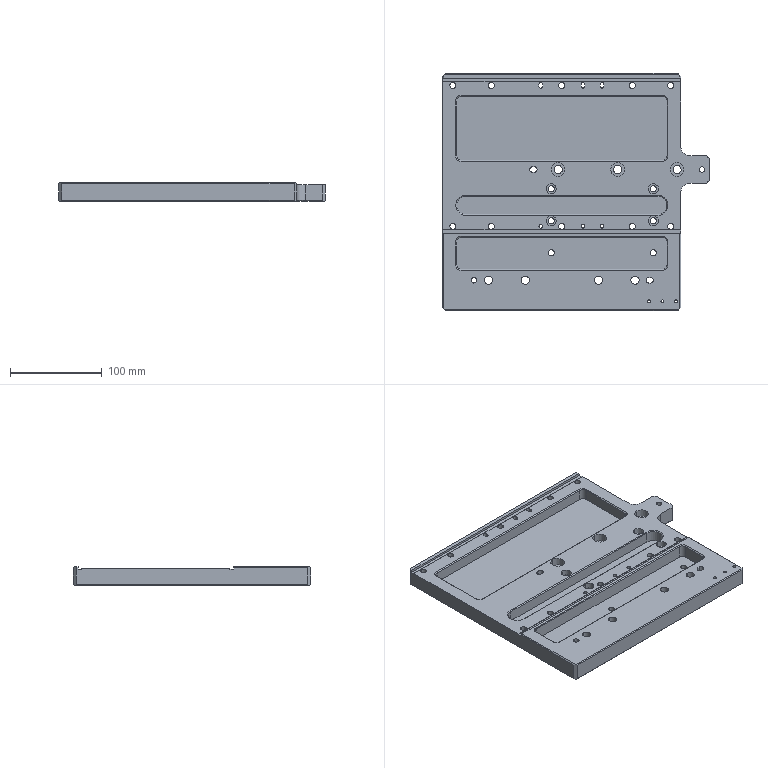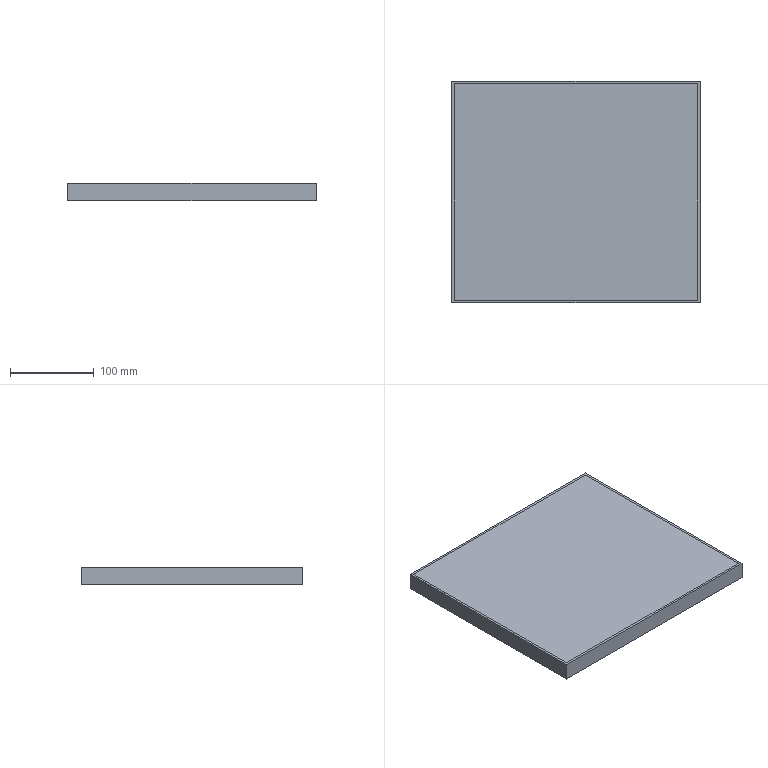CAM job | NX | 3-axis milling, drilling | part box 291 x 259 x 20 mm | stock box 297 x 265 x 21 mm
Tools:
number,name,description,diameter,corner_radius,flute_length,length,flutes
1,D50,Milling Tool-5 Parameters,50.0,0.0,50.0,75.0,2
3,D10,Milling Tool-5 Parameters,10.0,0.0,50.0,75.0,2
2,D6A45,Milling Tool-5 Parameters,6.0,0.0,3.0,3.0,2
12,3.8ZT,Drilling Tool,3.8,0.0,35.0,50.0,2
11,4.0JD,Milling Tool-5 Parameters,4.0,0.0,30.0,30.0,4
14,5.8ZT,Drilling Tool,5.8,0.0,35.0,50.0,2
16,6.0JD,Milling Tool-5 Parameters,6.0,0.0,30.0,30.0,4
17,6.6ZT,Drilling Tool,6.6,0.0,35.0,50.0,2
19,9.0ZT,Drilling Tool,9.0,0.0,35.0,50.0,2
13,3.3ZT,Drilling Tool,3.3,0.0,35.0,50.0,2
4,D10JING,Milling Tool-5 Parameters,10.0,0.0,50.0,75.0,2
8,D6,Milling Tool-5 Parameters,6.0,0.0,50.0,75.0,2
10,D4,Milling Tool-5 Parameters,4.0,0.0,50.0,75.0,2
20,D3,Milling Tool-5 Parameters,3.0,0.0,50.0,75.0,2
6,D8JING,Milling Tool-5 Parameters,8.0,0.0,50.0,75.0,2
Operations:
program,operation,operation_type,tool,method,geometry_group,spindle_rpm,surface_speed,feed_per_tooth,feed_cut,feed_plunge,cut_length_mm,path_length_mm,cut_time_min,machine_time_min
1-294-262-20AB胶,FLOOR_WALL,VolumeBased25DMillingOperation,D50,METHOD,A,6500.0,1286.0,0.0962,1250.0,100.0,4073.997,4127.997,3.259,3.265
1-294-262-20AB胶,ADAPTIVE_MILLING,CavityMilling,D10,METHOD,A,7000.0,219.0,0.2143,3000.0,1000.0,110241.217,126958.41,38.912,40.584
1-294-262-20AB胶,DRILLING_COPY_1,Operation,D6A45,METHOD,A,3000.0,56.0,0.0333,200.0,0.0,144.0,1687.131,0.72,0.8743
1-294-262-20AB胶,DRILLING_COPY_1_COPY_COPY_COPY_COPY_COPY,Operation,3.3ZT,METHOD,A,2000.0,20.0,0.0375,150.0,0.0,76.474,249.543,0.5098,0.5271
1-294-262-20AB胶,DRILLING_COPY_1_COPY_COPY_COPY_COPY_COPY_COPY_1,Operation,3.8ZT,METHOD,A,2000.0,20.0,0.0375,150.0,0.0,141.85,652.351,0.9457,0.9967
1-294-262-20AB胶,DRILLING_COPY_1_COPY_COPY_COPY_COPY_COPY_COPY_1_COPY,Operation,4.0JD,METHOD,A,1000.0,12.0,0.01,40.0,0.0,64.5,266.311,1.613,1.633
1-294-262-20AB胶,DRILLING_COPY_1_COPY_COPY_COPY_COPY_COPY_COPY_1_COPY_1,Operation,5.8ZT,METHOD,A,2000.0,20.0,0.0375,150.0,0.0,100.97,719.498,0.6731,0.735
1-294-262-20AB胶,DRILLING_COPY_1_COPY_COPY_COPY_COPY_COPY_COPY_1_COPY_1_COPY,Operation,6.0JD,METHOD,A,1000.0,15.0,0.01,40.0,0.0,45.0,431.845,1.125,1.164
1-294-262-20AB胶,DRILLING_COPY_1_COPY_COPY_COPY_COPY_COPY_COPY_1_COPY_1_COPY_1,Operation,6.6ZT,METHOD,A,2000.0,20.0,0.0375,150.0,0.0,357.725,1618.987,2.385,2.511
1-294-262-20AB胶,DRILLING_COPY_1_COPY_COPY_COPY_COPY_COPY_COPY_1_COPY_1_COPY_1_COPY,Operation,9.0ZT,METHOD,A,2000.0,20.0,0.0375,150.0,0.0,180.927,861.726,1.206,1.274
1-294-262-20AB胶,ZLEVEL_PROFILE,ZLevelMilling,D10,METHOD,A,7000.0,219.0,0.2143,3000.0,1000.0,22362.748,22439.147,7.486,7.493
1-294-262-20AB胶,FLOOR_WALL_1_COPY_1,VolumeBased25DMillingOperation,D10JING,METHOD,A,7000.0,87.0,0.0714,1000.0,100.0,16353.512,17764.561,16.354,16.515
1-294-262-20AB胶,HOLE_MILLING,CylinderMilling,D6,METHOD,A,7000.0,131.0,0.1071,1500.0,100.0,2633.021,3418.843,1.755,1.834
1-294-262-20AB胶,ZLEVEL_PROFILE_1_COPY_COPY,ZLevelMilling,D4,METHOD,A,7000.0,87.0,0.0929,1300.0,1000.0,1399.75,1730.901,1.088,1.121
1-294-262-20AB胶,ZLEVEL_PROFILE_1_COPY_COPY_COPY,ZLevelMilling,D3,METHOD,A,7000.0,65.0,0.0786,1100.0,1000.0,2119.398,2423.229,1.934,1.964
1-294-262-20AB胶,ZLEVEL_PROFILE_1_COPY_COPY_COPY_COPY,ZLevelMilling,D3,METHOD,A,7000.0,65.0,0.0786,1100.0,1000.0,3180.724,3612.601,2.893,2.936
1-294-262-20AB胶,ZLEVEL_PROFILE_COPY_1_COPY_COPY_COPY_COPY_2_COPY,ZLevelMilling,D6A45,METHOD,A,7000.0,131.0,0.0714,1000.0,1000.0,1885.481,4097.94,1.885,2.107
1-294-262-20AB胶,ZLEVEL_PROFILE_COPY_1_COPY_COPY_COPY_COPY_2_COPY_COPY,ZLevelMilling,D6A45,METHOD,A,7000.0,131.0,0.0714,1000.0,1000.0,1924.12,7369.493,1.924,2.469
1-294-262-20AB胶,刀补10,ZLevelMilling,D4,METHOD,A,7000.0,87.0,0.0571,800.0,1000.0,430.623,766.828,0.5377,0.5713
1-294-262-20AB胶,刀补10_COPY,ZLevelMilling,D3,METHOD,A,7000.0,87.0,0.0571,800.0,1000.0,450.023,757.54,0.5617,0.5925
1-294-262-20AB胶,刀补3,ZLevelMilling,D3,METHOD,A,7000.0,65.0,0.0571,800.0,1000.0,1063.262,1634.878,1.327,1.385
1-294-262-20AB胶,ZLEVEL_PROFILE_COPY_1_1,ZLevelMilling,D8JING,METHOD,A,7000.0,219.0,0.0714,1000.0,1000.0,3330.25,3427.85,3.33,3.34
2-294-262-20AB胶,FLOOR_WALL_COPY,VolumeBased25DMillingOperation,D50,METHOD,B,6500.0,1286.0,0.0962,1250.0,100.0,3746.711,3800.711,2.997,3.003
2-294-262-20AB胶,HOLE_MILLING_COPY,CylinderMilling,D6,METHOD,B,7000.0,131.0,0.1071,1500.0,100.0,4798.684,6550.799,3.199,3.374
2-294-262-20AB胶,ZLEVEL_PROFILE_COPY_1_COPY_COPY_COPY_COPY_2_COPY_COPY_1,ZLevelMilling,D6A45,METHOD,B,7000.0,131.0,0.0714,1000.0,1000.0,1825.104,8383.747,1.825,2.481